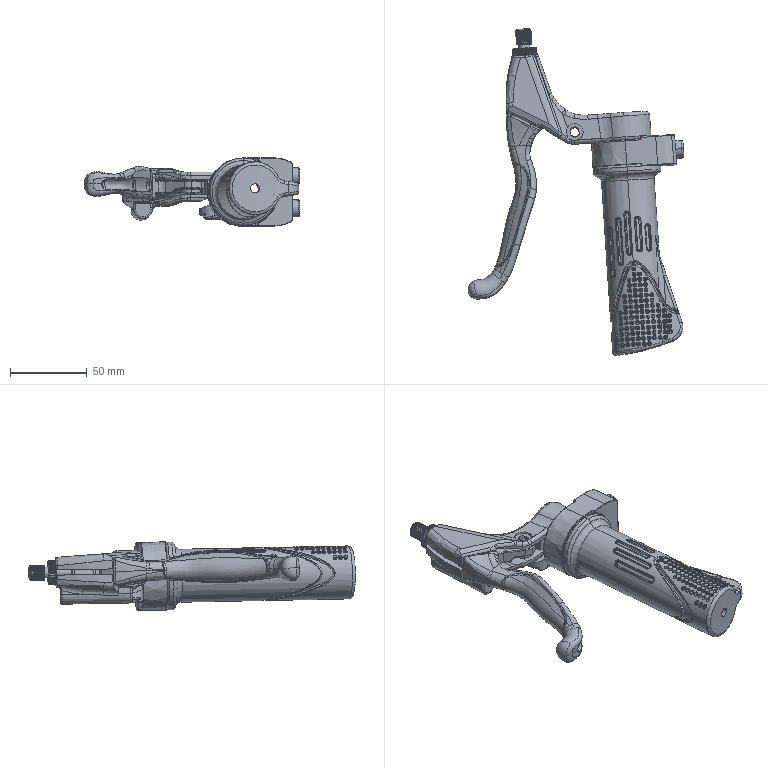Part | SolidWorks | features BaseBody 1 | 1 solid | 1865 faces | box 140.406 x 212.588 x 44.525 mm | volume 142694 mm3 | spline 893 | cylinder 649 | plane 196 | cone 63 | torus 57 | sphere 7 | commonest cylinder face diameters 2 x131 32.5 x114 0.6 x91 16 x34 2.24 x32 1.12 x30